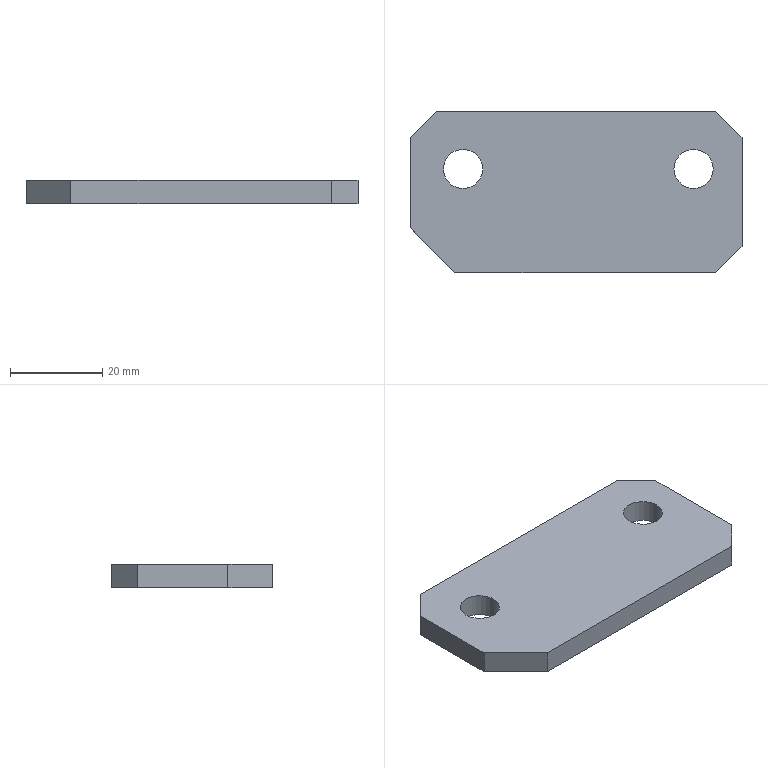Part | STEP file | gslz 2016.10.28-13_id1694_x_t | 1 solid | 12 faces | box 72 x 35 x 5 mm | volume 11553 mm3 | plane 10 | cylinder 2 | commonest cylinder face diameters 8.5 x2
STEP:
#1=CARTESIAN_POINT('',(0.,0.,0.));
#2=DIRECTION('',(0.,0.,1.));
#3=DIRECTION('',(1.,0.,0.));
#4=AXIS2_PLACEMENT_3D('',#1,#2,#3);
#5=CARTESIAN_POINT('',(516.464,-12.393,-94.));
#6=VERTEX_POINT('',#5);
#7=CARTESIAN_POINT('',(573.05,-12.393,-94.));
#8=VERTEX_POINT('',#7);
#9=CARTESIAN_POINT('',(-151.191,-12.393,-94.));
#10=DIRECTION('',(1.,0.,0.));
#11=VECTOR('',#10,1.);
#12=LINE('',#9,#11);
#13=CARTESIAN_POINT('',(-151.191,-12.393,-99.));
#14=DIRECTION('',(0.,-1.,0.));
#15=DIRECTION('',(0.,0.,-1.));
#16=AXIS2_PLACEMENT_3D('',#13,#14,#15);
#17=PLANE('',#16);
#18=CARTESIAN_POINT('',(-5.,0.));
#19=DIRECTION('',(0.,1.));
#20=VECTOR('',#19,1.);
#21=LINE('',#18,#20);
#22=(GEOMETRIC_REPRESENTATION_CONTEXT(2)PARAMETRIC_REPRESENTATION_CONTEXT()REPRESENTATION_CONTEXT('',''));
#23=DEFINITIONAL_REPRESENTATION('',(#21),#22);
#24=PCURVE('',#17,#23);
#25=CARTESIAN_POINT('',(-151.191,33.107,-94.));
#26=DIRECTION('',(0.,0.,-1.));
#27=DIRECTION('',(-1.,0.,0.));
#28=AXIS2_PLACEMENT_3D('',#25,#26,#27);
#29=PLANE('',#28);
#30=CARTESIAN_POINT('',(0.,-45.5));
#31=DIRECTION('',(-1.,0.));
#32=VECTOR('',#31,1.);
#33=LINE('',#30,#32);
#34=(GEOMETRIC_REPRESENTATION_CONTEXT(2)PARAMETRIC_REPRESENTATION_CONTEXT()REPRESENTATION_CONTEXT('',''));
#35=DEFINITIONAL_REPRESENTATION('',(#33),#34);
#36=PCURVE('',#29,#35);
#37=SURFACE_CURVE('',#12,(#24,#36),.PCURVE_S1.);
#38=EDGE_CURVE('',#6,#8,#37,.T.);
#39=ORIENTED_EDGE('',*,*,#38,.F.);
#40=CARTESIAN_POINT('',(516.464,-12.393,-99.));
#41=VERTEX_POINT('',#40);
#42=CARTESIAN_POINT('',(516.464,-12.393,-99.));
#43=DIRECTION('',(0.,0.,-1.));
#44=VECTOR('',#43,1.);
#45=LINE('',#42,#44);
#46=CARTESIAN_POINT('',(0.,667.655));
#47=DIRECTION('',(1.,0.));
#48=VECTOR('',#47,1.);
#49=LINE('',#46,#48);
#50=(GEOMETRIC_REPRESENTATION_CONTEXT(2)PARAMETRIC_REPRESENTATION_CONTEXT()REPRESENTATION_CONTEXT('',''));
#51=DEFINITIONAL_REPRESENTATION('',(#49),#50);
#52=PCURVE('',#17,#51);
#53=CARTESIAN_POINT('',(506.611,-2.54,-99.));
#54=DIRECTION('',(0.7071,0.7071,0.));
#55=DIRECTION('',(0.,0.,1.));
#56=AXIS2_PLACEMENT_3D('',#53,#54,#55);
#57=PLANE('',#56);
#58=CARTESIAN_POINT('',(0.,13.935));
#59=DIRECTION('',(-1.,0.));
#60=VECTOR('',#59,1.);
#61=LINE('',#58,#60);
#62=(GEOMETRIC_REPRESENTATION_CONTEXT(2)PARAMETRIC_REPRESENTATION_CONTEXT()REPRESENTATION_CONTEXT('',''));
#63=DEFINITIONAL_REPRESENTATION('',(#61),#62);
#64=PCURVE('',#57,#63);
#65=SURFACE_CURVE('',#45,(#52,#64),.PCURVE_S1.);
#66=EDGE_CURVE('',#6,#41,#65,.T.);
#67=ORIENTED_EDGE('',*,*,#66,.T.);
#68=CARTESIAN_POINT('',(573.05,-12.393,-99.));
#69=VERTEX_POINT('',#68);
#70=CARTESIAN_POINT('',(-151.191,-12.393,-99.));
#71=DIRECTION('',(1.,0.,0.));
#72=VECTOR('',#71,1.);
#73=LINE('',#70,#72);
#74=CARTESIAN_POINT('',(0.,0.));
#75=DIRECTION('',(0.,1.));
#76=VECTOR('',#75,1.);
#77=LINE('',#74,#76);
#78=(GEOMETRIC_REPRESENTATION_CONTEXT(2)PARAMETRIC_REPRESENTATION_CONTEXT()REPRESENTATION_CONTEXT('',''));
#79=DEFINITIONAL_REPRESENTATION('',(#77),#78);
#80=PCURVE('',#17,#79);
#81=CARTESIAN_POINT('',(-151.191,33.107,-99.));
#82=DIRECTION('',(0.,0.,-1.));
#83=DIRECTION('',(-1.,0.,0.));
#84=AXIS2_PLACEMENT_3D('',#81,#82,#83);
#85=PLANE('',#84);
#86=CARTESIAN_POINT('',(0.,-45.5));
#87=DIRECTION('',(-1.,0.));
#88=VECTOR('',#87,1.);
#89=LINE('',#86,#88);
#90=(GEOMETRIC_REPRESENTATION_CONTEXT(2)PARAMETRIC_REPRESENTATION_CONTEXT()REPRESENTATION_CONTEXT('',''));
#91=DEFINITIONAL_REPRESENTATION('',(#89),#90);
#92=PCURVE('',#85,#91);
#93=SURFACE_CURVE('',#73,(#80,#92),.PCURVE_S1.);
#94=EDGE_CURVE('',#41,#69,#93,.T.);
#95=ORIENTED_EDGE('',*,*,#94,.T.);
#96=CARTESIAN_POINT('',(573.05,-12.393,-99.));
#97=DIRECTION('',(0.,0.,1.));
#98=VECTOR('',#97,1.);
#99=LINE('',#96,#98);
#100=CARTESIAN_POINT('',(0.,724.241));
#101=DIRECTION('',(-1.,0.));
#102=VECTOR('',#101,1.);
#103=LINE('',#100,#102);
#104=(GEOMETRIC_REPRESENTATION_CONTEXT(2)PARAMETRIC_REPRESENTATION_CONTEXT()REPRESENTATION_CONTEXT('',''));
#105=DEFINITIONAL_REPRESENTATION('',(#103),#104);
#106=PCURVE('',#17,#105);
#107=CARTESIAN_POINT('',(572.904,-12.54,-99.));
#108=DIRECTION('',(0.7071,-0.7071,0.));
#109=DIRECTION('',(0.,0.,-1.));
#110=AXIS2_PLACEMENT_3D('',#107,#108,#109);
#111=PLANE('',#110);
#112=CARTESIAN_POINT('',(0.,0.2071));
#113=DIRECTION('',(-1.,0.));
#114=VECTOR('',#113,1.);
#115=LINE('',#112,#114);
#116=(GEOMETRIC_REPRESENTATION_CONTEXT(2)PARAMETRIC_REPRESENTATION_CONTEXT()REPRESENTATION_CONTEXT('',''));
#117=DEFINITIONAL_REPRESENTATION('',(#115),#116);
#118=PCURVE('',#111,#117);
#119=SURFACE_CURVE('',#99,(#106,#118),.PCURVE_S1.);
#120=EDGE_CURVE('',#69,#8,#119,.T.);
#121=ORIENTED_EDGE('',*,*,#120,.T.);
#122=EDGE_LOOP('',(#39,#67,#95,#121));
#123=FACE_BOUND('',#122,.T.);
#124=ADVANCED_FACE('',(#123),#17,.T.);
#125=CARTESIAN_POINT('',(506.757,16.9,-99.));
#126=VERTEX_POINT('',#125);
#127=CARTESIAN_POINT('',(506.757,-2.686,-99.));
#128=VERTEX_POINT('',#127);
#129=CARTESIAN_POINT('',(506.757,33.107,-99.));
#130=DIRECTION('',(0.,-1.,0.));
#131=VECTOR('',#130,1.);
#132=LINE('',#129,#131);
#133=CARTESIAN_POINT('',(506.757,33.107,-99.));
#134=DIRECTION('',(-1.,0.,0.));
#135=DIRECTION('',(0.,0.,1.));
#136=AXIS2_PLACEMENT_3D('',#133,#134,#135);
#137=PLANE('',#136);
#138=CARTESIAN_POINT('',(0.,0.));
#139=DIRECTION('',(0.,-1.));
#140=VECTOR('',#139,1.);
#141=LINE('',#138,#140);
#142=(GEOMETRIC_REPRESENTATION_CONTEXT(2)PARAMETRIC_REPRESENTATION_CONTEXT()REPRESENTATION_CONTEXT('',''));
#143=DEFINITIONAL_REPRESENTATION('',(#141),#142);
#144=PCURVE('',#137,#143);
#145=CARTESIAN_POINT('',(-657.948,0.));
#146=DIRECTION('',(0.,-1.));
#147=VECTOR('',#146,1.);
#148=LINE('',#145,#147);
#149=(GEOMETRIC_REPRESENTATION_CONTEXT(2)PARAMETRIC_REPRESENTATION_CONTEXT()REPRESENTATION_CONTEXT('',''));
#150=DEFINITIONAL_REPRESENTATION('',(#148),#149);
#151=PCURVE('',#85,#150);
#152=SURFACE_CURVE('',#132,(#144,#151),.PCURVE_S1.);
#153=EDGE_CURVE('',#126,#128,#152,.T.);
#154=ORIENTED_EDGE('',*,*,#153,.T.);
#155=CARTESIAN_POINT('',(506.757,-2.686,-94.));
#156=VERTEX_POINT('',#155);
#157=CARTESIAN_POINT('',(506.757,-2.686,-99.));
#158=DIRECTION('',(0.,0.,1.));
#159=VECTOR('',#158,1.);
#160=LINE('',#157,#159);
#161=CARTESIAN_POINT('',(0.,-35.793));
#162=DIRECTION('',(1.,0.));
#163=VECTOR('',#162,1.);
#164=LINE('',#161,#163);
#165=(GEOMETRIC_REPRESENTATION_CONTEXT(2)PARAMETRIC_REPRESENTATION_CONTEXT()REPRESENTATION_CONTEXT('',''));
#166=DEFINITIONAL_REPRESENTATION('',(#164),#165);
#167=PCURVE('',#137,#166);
#168=CARTESIAN_POINT('',(0.,0.2071));
#169=DIRECTION('',(1.,0.));
#170=VECTOR('',#169,1.);
#171=LINE('',#168,#170);
#172=(GEOMETRIC_REPRESENTATION_CONTEXT(2)PARAMETRIC_REPRESENTATION_CONTEXT()REPRESENTATION_CONTEXT('',''));
#173=DEFINITIONAL_REPRESENTATION('',(#171),#172);
#174=PCURVE('',#57,#173);
#175=SURFACE_CURVE('',#160,(#167,#174),.PCURVE_S1.);
#176=EDGE_CURVE('',#128,#156,#175,.T.);
#177=ORIENTED_EDGE('',*,*,#176,.T.);
#178=CARTESIAN_POINT('',(506.757,16.9,-94.));
#179=VERTEX_POINT('',#178);
#180=CARTESIAN_POINT('',(506.757,33.107,-94.));
#181=DIRECTION('',(0.,-1.,0.));
#182=VECTOR('',#181,1.);
#183=LINE('',#180,#182);
#184=CARTESIAN_POINT('',(5.,0.));
#185=DIRECTION('',(0.,-1.));
#186=VECTOR('',#185,1.);
#187=LINE('',#184,#186);
#188=(GEOMETRIC_REPRESENTATION_CONTEXT(2)PARAMETRIC_REPRESENTATION_CONTEXT()REPRESENTATION_CONTEXT('',''));
#189=DEFINITIONAL_REPRESENTATION('',(#187),#188);
#190=PCURVE('',#137,#189);
#191=CARTESIAN_POINT('',(-657.948,0.));
#192=DIRECTION('',(0.,-1.));
#193=VECTOR('',#192,1.);
#194=LINE('',#191,#193);
#195=(GEOMETRIC_REPRESENTATION_CONTEXT(2)PARAMETRIC_REPRESENTATION_CONTEXT()REPRESENTATION_CONTEXT('',''));
#196=DEFINITIONAL_REPRESENTATION('',(#194),#195);
#197=PCURVE('',#29,#196);
#198=SURFACE_CURVE('',#183,(#190,#197),.PCURVE_S1.);
#199=EDGE_CURVE('',#179,#156,#198,.T.);
#200=ORIENTED_EDGE('',*,*,#199,.F.);
#201=CARTESIAN_POINT('',(506.757,16.9,-99.));
#202=DIRECTION('',(0.,0.,-1.));
#203=VECTOR('',#202,1.);
#204=LINE('',#201,#203);
#205=CARTESIAN_POINT('',(0.,-16.207));
#206=DIRECTION('',(-1.,0.));
#207=VECTOR('',#206,1.);
#208=LINE('',#205,#207);
#209=(GEOMETRIC_REPRESENTATION_CONTEXT(2)PARAMETRIC_REPRESENTATION_CONTEXT()REPRESENTATION_CONTEXT('',''));
#210=DEFINITIONAL_REPRESENTATION('',(#208),#209);
#211=PCURVE('',#137,#210);
#212=CARTESIAN_POINT('',(512.611,22.753,-99.));
#213=DIRECTION('',(-0.7071,0.7071,0.));
#214=DIRECTION('',(0.,0.,-1.));
#215=AXIS2_PLACEMENT_3D('',#212,#213,#214);
#216=PLANE('',#215);
#217=CARTESIAN_POINT('',(0.,8.278));
#218=DIRECTION('',(1.,0.));
#219=VECTOR('',#218,1.);
#220=LINE('',#217,#219);
#221=(GEOMETRIC_REPRESENTATION_CONTEXT(2)PARAMETRIC_REPRESENTATION_CONTEXT()REPRESENTATION_CONTEXT('',''));
#222=DEFINITIONAL_REPRESENTATION('',(#220),#221);
#223=PCURVE('',#216,#222);
#224=SURFACE_CURVE('',#204,(#211,#223),.PCURVE_S1.);
#225=EDGE_CURVE('',#179,#126,#224,.T.);
#226=ORIENTED_EDGE('',*,*,#225,.T.);
#227=EDGE_LOOP('',(#154,#177,#200,#226));
#228=FACE_BOUND('',#227,.T.);
#229=ADVANCED_FACE('',(#228),#137,.T.);
#230=CARTESIAN_POINT('',(512.464,22.607,-94.));
#231=VERTEX_POINT('',#230);
#232=CARTESIAN_POINT('',(573.05,22.607,-94.));
#233=VERTEX_POINT('',#232);
#234=CARTESIAN_POINT('',(-151.191,22.607,-94.));
#235=DIRECTION('',(1.,0.,0.));
#236=VECTOR('',#235,1.);
#237=LINE('',#234,#236);
#238=CARTESIAN_POINT('',(-151.191,22.607,-99.));
#239=DIRECTION('',(0.,-1.,0.));
#240=DIRECTION('',(0.,0.,-1.));
#241=AXIS2_PLACEMENT_3D('',#238,#239,#240);
#242=PLANE('',#241);
#243=CARTESIAN_POINT('',(-5.,0.));
#244=DIRECTION('',(0.,1.));
#245=VECTOR('',#244,1.);
#246=LINE('',#243,#245);
#247=(GEOMETRIC_REPRESENTATION_CONTEXT(2)PARAMETRIC_REPRESENTATION_CONTEXT()REPRESENTATION_CONTEXT('',''));
#248=DEFINITIONAL_REPRESENTATION('',(#246),#247);
#249=PCURVE('',#242,#248);
#250=CARTESIAN_POINT('',(0.,-10.5));
#251=DIRECTION('',(-1.,0.));
#252=VECTOR('',#251,1.);
#253=LINE('',#250,#252);
#254=(GEOMETRIC_REPRESENTATION_CONTEXT(2)PARAMETRIC_REPRESENTATION_CONTEXT()REPRESENTATION_CONTEXT('',''));
#255=DEFINITIONAL_REPRESENTATION('',(#253),#254);
#256=PCURVE('',#29,#255);
#257=SURFACE_CURVE('',#237,(#249,#256),.PCURVE_S1.);
#258=EDGE_CURVE('',#231,#233,#257,.T.);
#259=ORIENTED_EDGE('',*,*,#258,.T.);
#260=CARTESIAN_POINT('',(573.05,22.607,-99.));
#261=VERTEX_POINT('',#260);
#262=CARTESIAN_POINT('',(573.05,22.607,-99.));
#263=DIRECTION('',(0.,0.,-1.));
#264=VECTOR('',#263,1.);
#265=LINE('',#262,#264);
#266=CARTESIAN_POINT('',(0.,724.241));
#267=DIRECTION('',(1.,0.));
#268=VECTOR('',#267,1.);
#269=LINE('',#266,#268);
#270=(GEOMETRIC_REPRESENTATION_CONTEXT(2)PARAMETRIC_REPRESENTATION_CONTEXT()REPRESENTATION_CONTEXT('',''));
#271=DEFINITIONAL_REPRESENTATION('',(#269),#270);
#272=PCURVE('',#242,#271);
#273=CARTESIAN_POINT('',(578.904,16.753,-99.));
#274=DIRECTION('',(-0.7071,-0.7071,0.));
#275=DIRECTION('',(0.,0.,1.));
#276=AXIS2_PLACEMENT_3D('',#273,#274,#275);
#277=PLANE('',#276);
#278=CARTESIAN_POINT('',(0.,8.278));
#279=DIRECTION('',(-1.,0.));
#280=VECTOR('',#279,1.);
#281=LINE('',#278,#280);
#282=(GEOMETRIC_REPRESENTATION_CONTEXT(2)PARAMETRIC_REPRESENTATION_CONTEXT()REPRESENTATION_CONTEXT('',''));
#283=DEFINITIONAL_REPRESENTATION('',(#281),#282);
#284=PCURVE('',#277,#283);
#285=SURFACE_CURVE('',#265,(#272,#284),.PCURVE_S1.);
#286=EDGE_CURVE('',#233,#261,#285,.T.);
#287=ORIENTED_EDGE('',*,*,#286,.T.);
#288=CARTESIAN_POINT('',(512.464,22.607,-99.));
#289=VERTEX_POINT('',#288);
#290=CARTESIAN_POINT('',(-151.191,22.607,-99.));
#291=DIRECTION('',(1.,0.,0.));
#292=VECTOR('',#291,1.);
#293=LINE('',#290,#292);
#294=CARTESIAN_POINT('',(0.,0.));
#295=DIRECTION('',(0.,1.));
#296=VECTOR('',#295,1.);
#297=LINE('',#294,#296);
#298=(GEOMETRIC_REPRESENTATION_CONTEXT(2)PARAMETRIC_REPRESENTATION_CONTEXT()REPRESENTATION_CONTEXT('',''));
#299=DEFINITIONAL_REPRESENTATION('',(#297),#298);
#300=PCURVE('',#242,#299);
#301=CARTESIAN_POINT('',(0.,-10.5));
#302=DIRECTION('',(-1.,0.));
#303=VECTOR('',#302,1.);
#304=LINE('',#301,#303);
#305=(GEOMETRIC_REPRESENTATION_CONTEXT(2)PARAMETRIC_REPRESENTATION_CONTEXT()REPRESENTATION_CONTEXT('',''));
#306=DEFINITIONAL_REPRESENTATION('',(#304),#305);
#307=PCURVE('',#85,#306);
#308=SURFACE_CURVE('',#293,(#300,#307),.PCURVE_S1.);
#309=EDGE_CURVE('',#289,#261,#308,.T.);
#310=ORIENTED_EDGE('',*,*,#309,.F.);
#311=CARTESIAN_POINT('',(512.464,22.607,-99.));
#312=DIRECTION('',(0.,0.,1.));
#313=VECTOR('',#312,1.);
#314=LINE('',#311,#313);
#315=CARTESIAN_POINT('',(0.,663.655));
#316=DIRECTION('',(-1.,0.));
#317=VECTOR('',#316,1.);
#318=LINE('',#315,#317);
#319=(GEOMETRIC_REPRESENTATION_CONTEXT(2)PARAMETRIC_REPRESENTATION_CONTEXT()REPRESENTATION_CONTEXT('',''));
#320=DEFINITIONAL_REPRESENTATION('',(#318),#319);
#321=PCURVE('',#242,#320);
#322=CARTESIAN_POINT('',(0.,0.2071));
#323=DIRECTION('',(-1.,0.));
#324=VECTOR('',#323,1.);
#325=LINE('',#322,#324);
#326=(GEOMETRIC_REPRESENTATION_CONTEXT(2)PARAMETRIC_REPRESENTATION_CONTEXT()REPRESENTATION_CONTEXT('',''));
#327=DEFINITIONAL_REPRESENTATION('',(#325),#326);
#328=PCURVE('',#216,#327);
#329=SURFACE_CURVE('',#314,(#321,#328),.PCURVE_S1.);
#330=EDGE_CURVE('',#289,#231,#329,.T.);
#331=ORIENTED_EDGE('',*,*,#330,.T.);
#332=EDGE_LOOP('',(#259,#287,#310,#331));
#333=FACE_BOUND('',#332,.T.);
#334=ADVANCED_FACE('',(#333),#242,.F.);
#335=CARTESIAN_POINT('',(514.007,10.107,-99.));
#336=VERTEX_POINT('',#335);
#337=CARTESIAN_POINT('',(518.257,10.107,-99.));
#338=DIRECTION('',(0.,0.,-1.));
#339=DIRECTION('',(-1.,0.,0.));
#340=AXIS2_PLACEMENT_3D('',#337,#338,#339);
#341=CIRCLE('',#340,4.25);
#342=CARTESIAN_POINT('',(518.257,10.107,-99.));
#343=DIRECTION('',(0.,0.,1.));
#344=DIRECTION('',(1.,0.,0.));
#345=AXIS2_PLACEMENT_3D('',#342,#343,#344);
#346=CYLINDRICAL_SURFACE('',#345,4.25);
#347=CARTESIAN_POINT('',(9.425,0.));
#348=DIRECTION('',(-1.,0.));
#349=VECTOR('',#348,1.);
#350=LINE('',#347,#349);
#351=(GEOMETRIC_REPRESENTATION_CONTEXT(2)PARAMETRIC_REPRESENTATION_CONTEXT()REPRESENTATION_CONTEXT('',''));
#352=DEFINITIONAL_REPRESENTATION('',(#350),#351);
#353=PCURVE('',#346,#352);
#354=CARTESIAN_POINT('',(-669.448,-23.));
#355=DIRECTION('',(1.,0.));
#356=AXIS2_PLACEMENT_2D('',#354,#355);
#357=CIRCLE('',#356,4.25);
#358=(GEOMETRIC_REPRESENTATION_CONTEXT(2)PARAMETRIC_REPRESENTATION_CONTEXT()REPRESENTATION_CONTEXT('',''));
#359=DEFINITIONAL_REPRESENTATION('',(#357),#358);
#360=PCURVE('',#85,#359);
#361=SURFACE_CURVE('',#341,(#353,#360),.PCURVE_S1.);
#362=EDGE_CURVE('',#336,#336,#361,.T.);
#363=ORIENTED_EDGE('',*,*,#362,.F.);
#364=CARTESIAN_POINT('',(514.007,10.107,-94.));
#365=VERTEX_POINT('',#364);
#366=CARTESIAN_POINT('',(514.007,10.107,-99.));
#367=CARTESIAN_POINT('',(514.007,10.107,-94.));
#368=B_SPLINE_CURVE_WITH_KNOTS('',1,(#366,#367),.UNSPECIFIED.,.F.,.F.,(2,2),(0.,5.),.PIECEWISE_BEZIER_KNOTS.);
#369=CARTESIAN_POINT('',(9.425,0.));
#370=DIRECTION('',(0.,1.));
#371=VECTOR('',#370,1.);
#372=LINE('',#369,#371);
#373=(GEOMETRIC_REPRESENTATION_CONTEXT(2)PARAMETRIC_REPRESENTATION_CONTEXT()REPRESENTATION_CONTEXT('',''));
#374=DEFINITIONAL_REPRESENTATION('',(#372),#373);
#375=PCURVE('',#346,#374);
#376=CARTESIAN_POINT('',(3.142,0.));
#377=DIRECTION('',(0.,1.));
#378=VECTOR('',#377,1.);
#379=LINE('',#376,#378);
#380=(GEOMETRIC_REPRESENTATION_CONTEXT(2)PARAMETRIC_REPRESENTATION_CONTEXT()REPRESENTATION_CONTEXT('',''));
#381=DEFINITIONAL_REPRESENTATION('',(#379),#380);
#382=PCURVE('',#346,#381);
#383=SEAM_CURVE('',#368,(#375,#382),.PCURVE_S1.);
#384=EDGE_CURVE('',#336,#365,#383,.T.);
#385=ORIENTED_EDGE('',*,*,#384,.T.);
#386=CARTESIAN_POINT('',(518.257,10.107,-94.));
#387=DIRECTION('',(0.,0.,-1.));
#388=DIRECTION('',(-1.,0.,0.));
#389=AXIS2_PLACEMENT_3D('',#386,#387,#388);
#390=CIRCLE('',#389,4.25);
#391=CARTESIAN_POINT('',(9.425,5.));
#392=DIRECTION('',(-1.,0.));
#393=VECTOR('',#392,1.);
#394=LINE('',#391,#393);
#395=(GEOMETRIC_REPRESENTATION_CONTEXT(2)PARAMETRIC_REPRESENTATION_CONTEXT()REPRESENTATION_CONTEXT('',''));
#396=DEFINITIONAL_REPRESENTATION('',(#394),#395);
#397=PCURVE('',#346,#396);
#398=CARTESIAN_POINT('',(-669.448,-23.));
#399=DIRECTION('',(1.,0.));
#400=AXIS2_PLACEMENT_2D('',#398,#399);
#401=CIRCLE('',#400,4.25);
#402=(GEOMETRIC_REPRESENTATION_CONTEXT(2)PARAMETRIC_REPRESENTATION_CONTEXT()REPRESENTATION_CONTEXT('',''));
#403=DEFINITIONAL_REPRESENTATION('',(#401),#402);
#404=PCURVE('',#29,#403);
#405=SURFACE_CURVE('',#390,(#397,#404),.PCURVE_S1.);
#406=EDGE_CURVE('',#365,#365,#405,.T.);
#407=ORIENTED_EDGE('',*,*,#406,.T.);
#408=ORIENTED_EDGE('',*,*,#384,.F.);
#409=EDGE_LOOP('',(#363,#385,#407,#408));
#410=FACE_BOUND('',#409,.F.);
#411=ADVANCED_FACE('',(#410),#346,.F.);
#412=CARTESIAN_POINT('',(564.007,10.107,-99.));
#413=VERTEX_POINT('',#412);
#414=CARTESIAN_POINT('',(568.257,10.107,-99.));
#415=DIRECTION('',(0.,0.,-1.));
#416=DIRECTION('',(-1.,0.,0.));
#417=AXIS2_PLACEMENT_3D('',#414,#415,#416);
#418=CIRCLE('',#417,4.25);
#419=CARTESIAN_POINT('',(568.257,10.107,-99.));
#420=DIRECTION('',(0.,0.,1.));
#421=DIRECTION('',(1.,0.,0.));
#422=AXIS2_PLACEMENT_3D('',#419,#420,#421);
#423=CYLINDRICAL_SURFACE('',#422,4.25);
#424=CARTESIAN_POINT('',(9.425,0.));
#425=DIRECTION('',(-1.,0.));
#426=VECTOR('',#425,1.);
#427=LINE('',#424,#426);
#428=(GEOMETRIC_REPRESENTATION_CONTEXT(2)PARAMETRIC_REPRESENTATION_CONTEXT()REPRESENTATION_CONTEXT('',''));
#429=DEFINITIONAL_REPRESENTATION('',(#427),#428);
#430=PCURVE('',#423,#429);
#431=CARTESIAN_POINT('',(-719.448,-23.));
#432=DIRECTION('',(1.,0.));
#433=AXIS2_PLACEMENT_2D('',#431,#432);
#434=CIRCLE('',#433,4.25);
#435=(GEOMETRIC_REPRESENTATION_CONTEXT(2)PARAMETRIC_REPRESENTATION_CONTEXT()REPRESENTATION_CONTEXT('',''));
#436=DEFINITIONAL_REPRESENTATION('',(#434),#435);
#437=PCURVE('',#85,#436);
#438=SURFACE_CURVE('',#418,(#430,#437),.PCURVE_S1.);
#439=EDGE_CURVE('',#413,#413,#438,.T.);
#440=ORIENTED_EDGE('',*,*,#439,.F.);
#441=CARTESIAN_POINT('',(564.007,10.107,-94.));
#442=VERTEX_POINT('',#441);
#443=CARTESIAN_POINT('',(564.007,10.107,-99.));
#444=CARTESIAN_POINT('',(564.007,10.107,-94.));
#445=B_SPLINE_CURVE_WITH_KNOTS('',1,(#443,#444),.UNSPECIFIED.,.F.,.F.,(2,2),(0.,5.),.PIECEWISE_BEZIER_KNOTS.);
#446=CARTESIAN_POINT('',(9.425,0.));
#447=DIRECTION('',(0.,1.));
#448=VECTOR('',#447,1.);
#449=LINE('',#446,#448);
#450=(GEOMETRIC_REPRESENTATION_CONTEXT(2)PARAMETRIC_REPRESENTATION_CONTEXT()REPRESENTATION_CONTEXT('',''));
#451=DEFINITIONAL_REPRESENTATION('',(#449),#450);
#452=PCURVE('',#423,#451);
#453=CARTESIAN_POINT('',(3.142,0.));
#454=DIRECTION('',(0.,1.));
#455=VECTOR('',#454,1.);
#456=LINE('',#453,#455);
#457=(GEOMETRIC_REPRESENTATION_CONTEXT(2)PARAMETRIC_REPRESENTATION_CONTEXT()REPRESENTATION_CONTEXT('',''));
#458=DEFINITIONAL_REPRESENTATION('',(#456),#457);
#459=PCURVE('',#423,#458);
#460=SEAM_CURVE('',#445,(#452,#459),.PCURVE_S1.);
#461=EDGE_CURVE('',#413,#442,#460,.T.);
#462=ORIENTED_EDGE('',*,*,#461,.T.);
#463=CARTESIAN_POINT('',(568.257,10.107,-94.));
#464=DIRECTION('',(0.,0.,-1.));
#465=DIRECTION('',(-1.,0.,0.));
#466=AXIS2_PLACEMENT_3D('',#463,#464,#465);
#467=CIRCLE('',#466,4.25);
#468=CARTESIAN_POINT('',(9.425,5.));
#469=DIRECTION('',(-1.,0.));
#470=VECTOR('',#469,1.);
#471=LINE('',#468,#470);
#472=(GEOMETRIC_REPRESENTATION_CONTEXT(2)PARAMETRIC_REPRESENTATION_CONTEXT()REPRESENTATION_CONTEXT('',''));
#473=DEFINITIONAL_REPRESENTATION('',(#471),#472);
#474=PCURVE('',#423,#473);
#475=CARTESIAN_POINT('',(-719.448,-23.));
#476=DIRECTION('',(1.,0.));
#477=AXIS2_PLACEMENT_2D('',#475,#476);
#478=CIRCLE('',#477,4.25);
#479=(GEOMETRIC_REPRESENTATION_CONTEXT(2)PARAMETRIC_REPRESENTATION_CONTEXT()REPRESENTATION_CONTEXT('',''));
#480=DEFINITIONAL_REPRESENTATION('',(#478),#479);
#481=PCURVE('',#29,#480);
#482=SURFACE_CURVE('',#467,(#474,#481),.PCURVE_S1.);
#483=EDGE_CURVE('',#442,#442,#482,.T.);
#484=ORIENTED_EDGE('',*,*,#483,.T.);
#485=ORIENTED_EDGE('',*,*,#461,.F.);
#486=EDGE_LOOP('',(#440,#462,#484,#485));
#487=FACE_BOUND('',#486,.F.);
#488=ADVANCED_FACE('',(#487),#423,.F.);
#489=CARTESIAN_POINT('',(578.757,16.9,-94.));
#490=VERTEX_POINT('',#489);
#491=CARTESIAN_POINT('',(578.757,-6.686,-94.));
#492=VERTEX_POINT('',#491);
#493=CARTESIAN_POINT('',(578.757,33.107,-94.));
#494=DIRECTION('',(0.,-1.,0.));
#495=VECTOR('',#494,1.);
#496=LINE('',#493,#495);
#497=CARTESIAN_POINT('',(578.757,33.107,-99.));
#498=DIRECTION('',(-1.,0.,0.));
#499=DIRECTION('',(0.,0.,1.));
#500=AXIS2_PLACEMENT_3D('',#497,#498,#499);
#501=PLANE('',#500);
#502=CARTESIAN_POINT('',(5.,0.));
#503=DIRECTION('',(0.,-1.));
#504=VECTOR('',#503,1.);
#505=LINE('',#502,#504);
#506=(GEOMETRIC_REPRESENTATION_CONTEXT(2)PARAMETRIC_REPRESENTATION_CONTEXT()REPRESENTATION_CONTEXT('',''));
#507=DEFINITIONAL_REPRESENTATION('',(#505),#506);
#508=PCURVE('',#501,#507);
#509=CARTESIAN_POINT('',(-729.948,0.));
#510=DIRECTION('',(0.,-1.));
#511=VECTOR('',#510,1.);
#512=LINE('',#509,#511);
#513=(GEOMETRIC_REPRESENTATION_CONTEXT(2)PARAMETRIC_REPRESENTATION_CONTEXT()REPRESENTATION_CONTEXT('',''));
#514=DEFINITIONAL_REPRESENTATION('',(#512),#513);
#515=PCURVE('',#29,#514);
#516=SURFACE_CURVE('',#496,(#508,#515),.PCURVE_S1.);
#517=EDGE_CURVE('',#490,#492,#516,.T.);
#518=ORIENTED_EDGE('',*,*,#517,.T.);
#519=CARTESIAN_POINT('',(578.757,-6.686,-99.));
#520=VERTEX_POINT('',#519);
#521=CARTESIAN_POINT('',(578.757,-6.686,-99.));
#522=DIRECTION('',(0.,0.,-1.));
#523=VECTOR('',#522,1.);
#524=LINE('',#521,#523);
#525=CARTESIAN_POINT('',(0.,-39.793));
#526=DIRECTION('',(-1.,0.));
#527=VECTOR('',#526,1.);
#528=LINE('',#525,#527);
#529=(GEOMETRIC_REPRESENTATION_CONTEXT(2)PARAMETRIC_REPRESENTATION_CONTEXT()REPRESENTATION_CONTEXT('',''));
#530=DEFINITIONAL_REPRESENTATION('',(#528),#529);
#531=PCURVE('',#501,#530);
#532=CARTESIAN_POINT('',(0.,8.278));
#533=DIRECTION('',(1.,0.));
#534=VECTOR('',#533,1.);
#535=LINE('',#532,#534);
#536=(GEOMETRIC_REPRESENTATION_CONTEXT(2)PARAMETRIC_REPRESENTATION_CONTEXT()REPRESENTATION_CONTEXT('',''));
#537=DEFINITIONAL_REPRESENTATION('',(#535),#536);
#538=PCURVE('',#111,#537);
#539=SURFACE_CURVE('',#524,(#531,#538),.PCURVE_S1.);
#540=EDGE_CURVE('',#492,#520,#539,.T.);
#541=ORIENTED_EDGE('',*,*,#540,.T.);
#542=CARTESIAN_POINT('',(578.757,16.9,-99.));
#543=VERTEX_POINT('',#542);
#544=CARTESIAN_POINT('',(578.757,33.107,-99.));
#545=DIRECTION('',(0.,-1.,0.));
#546=VECTOR('',#545,1.);
#547=LINE('',#544,#546);
#548=CARTESIAN_POINT('',(0.,0.));
#549=DIRECTION('',(0.,-1.));
#550=VECTOR('',#549,1.);
#551=LINE('',#548,#550);
#552=(GEOMETRIC_REPRESENTATION_CONTEXT(2)PARAMETRIC_REPRESENTATION_CONTEXT()REPRESENTATION_CONTEXT('',''));
#553=DEFINITIONAL_REPRESENTATION('',(#551),#552);
#554=PCURVE('',#501,#553);
#555=CARTESIAN_POINT('',(-729.948,0.));
#556=DIRECTION('',(0.,-1.));
#557=VECTOR('',#556,1.);
#558=LINE('',#555,#557);
#559=(GEOMETRIC_REPRESENTATION_CONTEXT(2)PARAMETRIC_REPRESENTATION_CONTEXT()REPRESENTATION_CONTEXT('',''));
#560=DEFINITIONAL_REPRESENTATION('',(#558),#559);
#561=PCURVE('',#85,#560);
#562=SURFACE_CURVE('',#547,(#554,#561),.PCURVE_S1.);
#563=EDGE_CURVE('',#543,#520,#562,.T.);
#564=ORIENTED_EDGE('',*,*,#563,.F.);
#565=CARTESIAN_POINT('',(578.757,16.9,-99.));
#566=DIRECTION('',(0.,0.,1.));
#567=VECTOR('',#566,1.);
#568=LINE('',#565,#567);
#569=CARTESIAN_POINT('',(0.,-16.207));
#570=DIRECTION('',(1.,0.));
#571=VECTOR('',#570,1.);
#572=LINE('',#569,#571);
#573=(GEOMETRIC_REPRESENTATION_CONTEXT(2)PARAMETRIC_REPRESENTATION_CONTEXT()REPRESENTATION_CONTEXT('',''));
#574=DEFINITIONAL_REPRESENTATION('',(#572),#573);
#575=PCURVE('',#501,#574);
#576=CARTESIAN_POINT('',(0.,0.2071));
#577=DIRECTION('',(1.,0.));
#578=VECTOR('',#577,1.);
#579=LINE('',#576,#578);
#580=(GEOMETRIC_REPRESENTATION_CONTEXT(2)PARAMETRIC_REPRESENTATION_CONTEXT()REPRESENTATION_CONTEXT('',''));
#581=DEFINITIONAL_REPRESENTATION('',(#579),#580);
#582=PCURVE('',#277,#581);
#583=SURFACE_CURVE('',#568,(#575,#582),.PCURVE_S1.);
#584=EDGE_CURVE('',#543,#490,#583,.T.);
#585=ORIENTED_EDGE('',*,*,#584,.T.);
#586=EDGE_LOOP('',(#518,#541,#564,#585));
#587=FACE_BOUND('',#586,.T.);
#588=ADVANCED_FACE('',(#587),#501,.F.);
#589=ORIENTED_EDGE('',*,*,#439,.F.);
#590=EDGE_LOOP('',(#589));
#591=FACE_BOUND('',#590,.T.);
#592=ORIENTED_EDGE('',*,*,#362,.F.);
#593=EDGE_LOOP('',(#592));
#594=FACE_BOUND('',#593,.T.);
#595=ORIENTED_EDGE('',*,*,#94,.F.);
#596=CARTESIAN_POINT('',(162.887,341.184,-99.));
#597=DIRECTION('',(-0.7071,0.7071,0.));
#598=VECTOR('',#597,1.);
#599=LINE('',#596,#598);
#600=CARTESIAN_POINT('',(-314.077,308.077));
#601=DIRECTION('',(0.7071,0.7071));
#602=VECTOR('',#601,1.);
#603=LINE('',#600,#602);
#604=(GEOMETRIC_REPRESENTATION_CONTEXT(2)PARAMETRIC_REPRESENTATION_CONTEXT()REPRESENTATION_CONTEXT('',''));
#605=DEFINITIONAL_REPRESENTATION('',(#603),#604);
#606=PCURVE('',#85,#605);
#607=CARTESIAN_POINT('',(0.,-486.099));
#608=DIRECTION('',(0.,-1.));
#609=VECTOR('',#608,1.);
#610=LINE('',#607,#609);
#611=(GEOMETRIC_REPRESENTATION_CONTEXT(2)PARAMETRIC_REPRESENTATION_CONTEXT()REPRESENTATION_CONTEXT('',''));
#612=DEFINITIONAL_REPRESENTATION('',(#610),#611);
#613=PCURVE('',#57,#612);
#614=SURFACE_CURVE('',#599,(#606,#613),.PCURVE_S1.);
#615=EDGE_CURVE('',#41,#128,#614,.T.);
#616=ORIENTED_EDGE('',*,*,#615,.T.);
#617=ORIENTED_EDGE('',*,*,#153,.F.);
#618=CARTESIAN_POINT('',(185.887,-303.971,-99.));
#619=DIRECTION('',(0.7071,0.7071,0.));
#620=VECTOR('',#619,1.);
#621=LINE('',#618,#620);
#622=CARTESIAN_POINT('',(-337.077,-337.077));
#623=DIRECTION('',(-0.7071,0.7071));
#624=VECTOR('',#623,1.);
#625=LINE('',#622,#624);
#626=(GEOMETRIC_REPRESENTATION_CONTEXT(2)PARAMETRIC_REPRESENTATION_CONTEXT()REPRESENTATION_CONTEXT('',''));
#627=DEFINITIONAL_REPRESENTATION('',(#625),#626);
#628=PCURVE('',#85,#627);
#629=CARTESIAN_POINT('',(0.,462.057));
#630=DIRECTION('',(0.,-1.));
#631=VECTOR('',#630,1.);
#632=LINE('',#629,#631);
#633=(GEOMETRIC_REPRESENTATION_CONTEXT(2)PARAMETRIC_REPRESENTATION_CONTEXT()REPRESENTATION_CONTEXT('',''));
#634=DEFINITIONAL_REPRESENTATION('',(#632),#633);
#635=PCURVE('',#216,#634);
#636=SURFACE_CURVE('',#621,(#628,#635),.PCURVE_S1.);
#637=EDGE_CURVE('',#126,#289,#636,.T.);
#638=ORIENTED_EDGE('',*,*,#637,.T.);
#639=ORIENTED_EDGE('',*,*,#309,.T.);
#640=CARTESIAN_POINT('',(205.68,389.977,-99.));
#641=DIRECTION('',(0.7071,-0.7071,0.));
#642=VECTOR('',#641,1.);
#643=LINE('',#640,#642);
#644=CARTESIAN_POINT('',(-356.87,356.87));
#645=DIRECTION('',(-0.7071,-0.7071));
#646=VECTOR('',#645,1.);
#647=LINE('',#644,#646);
#648=(GEOMETRIC_REPRESENTATION_CONTEXT(2)PARAMETRIC_REPRESENTATION_CONTEXT()REPRESENTATION_CONTEXT('',''));
#649=DEFINITIONAL_REPRESENTATION('',(#647),#648);
#650=PCURVE('',#85,#649);
#651=CARTESIAN_POINT('',(0.,527.818));
#652=DIRECTION('',(0.,-1.));
#653=VECTOR('',#652,1.);
#654=LINE('',#651,#653);
#655=(GEOMETRIC_REPRESENTATION_CONTEXT(2)PARAMETRIC_REPRESENTATION_CONTEXT()REPRESENTATION_CONTEXT('',''));
#656=DEFINITIONAL_REPRESENTATION('',(#654),#655);
#657=PCURVE('',#277,#656);
#658=SURFACE_CURVE('',#643,(#650,#657),.PCURVE_S1.);
#659=EDGE_CURVE('',#261,#543,#658,.T.);
#660=ORIENTED_EDGE('',*,*,#659,.T.);
#661=ORIENTED_EDGE('',*,*,#563,.T.);
#662=CARTESIAN_POINT('',(230.68,-354.764,-99.));
#663=DIRECTION('',(-0.7071,-0.7071,0.));
#664=VECTOR('',#663,1.);
#665=LINE('',#662,#664);
#666=CARTESIAN_POINT('',(-381.87,-387.87));
#667=DIRECTION('',(0.7071,-0.7071));
#668=VECTOR('',#667,1.);
#669=LINE('',#666,#668);
#670=(GEOMETRIC_REPRESENTATION_CONTEXT(2)PARAMETRIC_REPRESENTATION_CONTEXT()REPRESENTATION_CONTEXT('',''));
#671=DEFINITIONAL_REPRESENTATION('',(#669),#670);
#672=PCURVE('',#85,#671);
#673=CARTESIAN_POINT('',(0.,-483.978));
#674=DIRECTION('',(0.,-1.));
#675=VECTOR('',#674,1.);
#676=LINE('',#673,#675);
#677=(GEOMETRIC_REPRESENTATION_CONTEXT(2)PARAMETRIC_REPRESENTATION_CONTEXT()REPRESENTATION_CONTEXT('',''));
#678=DEFINITIONAL_REPRESENTATION('',(#676),#677);
#679=PCURVE('',#111,#678);
#680=SURFACE_CURVE('',#665,(#672,#679),.PCURVE_S1.);
#681=EDGE_CURVE('',#520,#69,#680,.T.);
#682=ORIENTED_EDGE('',*,*,#681,.T.);
#683=EDGE_LOOP('',(#595,#616,#617,#638,#639,#660,#661,#682));
#684=FACE_BOUND('',#683,.T.);
#685=ADVANCED_FACE('',(#591,#594,#684),#85,.T.);
#686=ORIENTED_EDGE('',*,*,#483,.T.);
#687=EDGE_LOOP('',(#686));
#688=FACE_BOUND('',#687,.T.);
#689=ORIENTED_EDGE('',*,*,#406,.T.);
#690=EDGE_LOOP('',(#689));
#691=FACE_BOUND('',#690,.T.);
#692=ORIENTED_EDGE('',*,*,#199,.T.);
#693=CARTESIAN_POINT('',(506.611,-2.54,-94.));
#694=DIRECTION('',(0.7071,-0.7071,0.));
#695=VECTOR('',#694,1.);
#696=LINE('',#693,#695);
#697=CARTESIAN_POINT('',(-657.801,-35.646));
#698=DIRECTION('',(-0.7071,-0.7071));
#699=VECTOR('',#698,1.);
#700=LINE('',#697,#699);
#701=(GEOMETRIC_REPRESENTATION_CONTEXT(2)PARAMETRIC_REPRESENTATION_CONTEXT()REPRESENTATION_CONTEXT('',''));
#702=DEFINITIONAL_REPRESENTATION('',(#700),#701);
#703=PCURVE('',#29,#702);
#704=CARTESIAN_POINT('',(5.,0.));
#705=DIRECTION('',(0.,1.));
#706=VECTOR('',#705,1.);
#707=LINE('',#704,#706);
#708=(GEOMETRIC_REPRESENTATION_CONTEXT(2)PARAMETRIC_REPRESENTATION_CONTEXT()REPRESENTATION_CONTEXT('',''));
#709=DEFINITIONAL_REPRESENTATION('',(#707),#708);
#710=PCURVE('',#57,#709);
#711=SURFACE_CURVE('',#696,(#703,#710),.PCURVE_S1.);
#712=EDGE_CURVE('',#156,#6,#711,.T.);
#713=ORIENTED_EDGE('',*,*,#712,.T.);
#714=ORIENTED_EDGE('',*,*,#38,.T.);
#715=CARTESIAN_POINT('',(572.904,-12.54,-94.));
#716=DIRECTION('',(0.7071,0.7071,0.));
#717=VECTOR('',#716,1.);
#718=LINE('',#715,#717);
#719=CARTESIAN_POINT('',(-724.094,-45.646));
#720=DIRECTION('',(-0.7071,0.7071));
#721=VECTOR('',#720,1.);
#722=LINE('',#719,#721);
#723=(GEOMETRIC_REPRESENTATION_CONTEXT(2)PARAMETRIC_REPRESENTATION_CONTEXT()REPRESENTATION_CONTEXT('',''));
#724=DEFINITIONAL_REPRESENTATION('',(#722),#723);
#725=PCURVE('',#29,#724);
#726=CARTESIAN_POINT('',(-5.,0.));
#727=DIRECTION('',(0.,1.));
#728=VECTOR('',#727,1.);
#729=LINE('',#726,#728);
#730=(GEOMETRIC_REPRESENTATION_CONTEXT(2)PARAMETRIC_REPRESENTATION_CONTEXT()REPRESENTATION_CONTEXT('',''));
#731=DEFINITIONAL_REPRESENTATION('',(#729),#730);
#732=PCURVE('',#111,#731);
#733=SURFACE_CURVE('',#718,(#725,#732),.PCURVE_S1.);
#734=EDGE_CURVE('',#8,#492,#733,.T.);
#735=ORIENTED_EDGE('',*,*,#734,.T.);
#736=ORIENTED_EDGE('',*,*,#517,.F.);
#737=CARTESIAN_POINT('',(578.904,16.753,-94.));
#738=DIRECTION('',(-0.7071,0.7071,0.));
#739=VECTOR('',#738,1.);
#740=LINE('',#737,#739);
#741=CARTESIAN_POINT('',(-730.094,-16.354));
#742=DIRECTION('',(0.7071,0.7071));
#743=VECTOR('',#742,1.);
#744=LINE('',#741,#743);
#745=(GEOMETRIC_REPRESENTATION_CONTEXT(2)PARAMETRIC_REPRESENTATION_CONTEXT()REPRESENTATION_CONTEXT('',''));
#746=DEFINITIONAL_REPRESENTATION('',(#744),#745);
#747=PCURVE('',#29,#746);
#748=CARTESIAN_POINT('',(5.,0.));
#749=DIRECTION('',(0.,1.));
#750=VECTOR('',#749,1.);
#751=LINE('',#748,#750);
#752=(GEOMETRIC_REPRESENTATION_CONTEXT(2)PARAMETRIC_REPRESENTATION_CONTEXT()REPRESENTATION_CONTEXT('',''));
#753=DEFINITIONAL_REPRESENTATION('',(#751),#752);
#754=PCURVE('',#277,#753);
#755=SURFACE_CURVE('',#740,(#747,#754),.PCURVE_S1.);
#756=EDGE_CURVE('',#490,#233,#755,.T.);
#757=ORIENTED_EDGE('',*,*,#756,.T.);
#758=ORIENTED_EDGE('',*,*,#258,.F.);
#759=CARTESIAN_POINT('',(512.611,22.753,-94.));
#760=DIRECTION('',(-0.7071,-0.7071,0.));
#761=VECTOR('',#760,1.);
#762=LINE('',#759,#761);
#763=CARTESIAN_POINT('',(-663.801,-10.354));
#764=DIRECTION('',(0.7071,-0.7071));
#765=VECTOR('',#764,1.);
#766=LINE('',#763,#765);
#767=(GEOMETRIC_REPRESENTATION_CONTEXT(2)PARAMETRIC_REPRESENTATION_CONTEXT()REPRESENTATION_CONTEXT('',''));
#768=DEFINITIONAL_REPRESENTATION('',(#766),#767);
#769=PCURVE('',#29,#768);
#770=CARTESIAN_POINT('',(-5.,0.));
#771=DIRECTION('',(0.,1.));
#772=VECTOR('',#771,1.);
#773=LINE('',#770,#772);
#774=(GEOMETRIC_REPRESENTATION_CONTEXT(2)PARAMETRIC_REPRESENTATION_CONTEXT()REPRESENTATION_CONTEXT('',''));
#775=DEFINITIONAL_REPRESENTATION('',(#773),#774);
#776=PCURVE('',#216,#775);
#777=SURFACE_CURVE('',#762,(#769,#776),.PCURVE_S1.);
#778=EDGE_CURVE('',#231,#179,#777,.T.);
#779=ORIENTED_EDGE('',*,*,#778,.T.);
#780=EDGE_LOOP('',(#692,#713,#714,#735,#736,#757,#758,#779));
#781=FACE_BOUND('',#780,.T.);
#782=ADVANCED_FACE('',(#688,#691,#781),#29,.F.);
#783=ORIENTED_EDGE('',*,*,#681,.F.);
#784=ORIENTED_EDGE('',*,*,#540,.F.);
#785=ORIENTED_EDGE('',*,*,#734,.F.);
#786=ORIENTED_EDGE('',*,*,#120,.F.);
#787=EDGE_LOOP('',(#783,#784,#785,#786));
#788=FACE_BOUND('',#787,.T.);
#789=ADVANCED_FACE('',(#788),#111,.T.);
#790=ORIENTED_EDGE('',*,*,#659,.F.);
#791=ORIENTED_EDGE('',*,*,#286,.F.);
#792=ORIENTED_EDGE('',*,*,#756,.F.);
#793=ORIENTED_EDGE('',*,*,#584,.F.);
#794=EDGE_LOOP('',(#790,#791,#792,#793));
#795=FACE_BOUND('',#794,.T.);
#796=ADVANCED_FACE('',(#795),#277,.F.);
#797=ORIENTED_EDGE('',*,*,#637,.F.);
#798=ORIENTED_EDGE('',*,*,#225,.F.);
#799=ORIENTED_EDGE('',*,*,#778,.F.);
#800=ORIENTED_EDGE('',*,*,#330,.F.);
#801=EDGE_LOOP('',(#797,#798,#799,#800));
#802=FACE_BOUND('',#801,.T.);
#803=ADVANCED_FACE('',(#802),#216,.T.);
#804=ORIENTED_EDGE('',*,*,#615,.F.);
#805=ORIENTED_EDGE('',*,*,#66,.F.);
#806=ORIENTED_EDGE('',*,*,#712,.F.);
#807=ORIENTED_EDGE('',*,*,#176,.F.);
#808=EDGE_LOOP('',(#804,#805,#806,#807));
#809=FACE_BOUND('',#808,.T.);
#810=ADVANCED_FACE('',(#809),#57,.F.);
#811=CLOSED_SHELL('',(#124,#229,#334,#411,#488,#588,#685,#782,#789,#796,#803,#810));
#812=MANIFOLD_SOLID_BREP('',#811);
#813=(LENGTH_UNIT()NAMED_UNIT(*)SI_UNIT(.MILLI.,.METRE.));
#814=UNCERTAINTY_MEASURE_WITH_UNIT(LENGTH_MEASURE(0.000002),#813,'','');
#815=(NAMED_UNIT(*)PLANE_ANGLE_UNIT()SI_UNIT($,.RADIAN.));
#816=(NAMED_UNIT(*)SI_UNIT($,.STERADIAN.)SOLID_ANGLE_UNIT());
#817=(GEOMETRIC_REPRESENTATION_CONTEXT(3)GLOBAL_UNCERTAINTY_ASSIGNED_CONTEXT((#814))GLOBAL_UNIT_ASSIGNED_CONTEXT((#813,#815,#816))REPRESENTATION_CONTEXT('',''));
#818=ADVANCED_BREP_SHAPE_REPRESENTATION('',(#4,#812),#817);